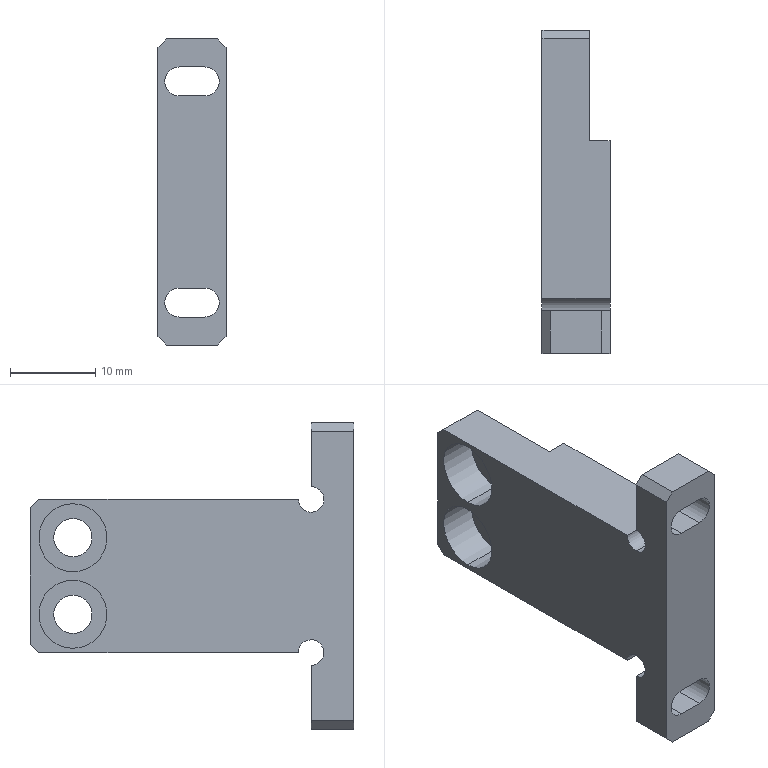Part | SolidWorks | features HoleWzd 2, ICE 2, Chamfer 1, Extrusion 1 | 1 solid | 39 faces | box 8 x 38 x 36 mm | volume 4843 mm3 | plane 24 | cylinder 15 | commonest cylinder face diameters 3.4 x4 4.5 x4 8 x4 3 x3
STEP:
#1=CARTESIAN_POINT('',(4.6,33.,-8.5));
#2=VERTEX_POINT('',#1);
#3=CARTESIAN_POINT('',(4.6,33.,-0.5));
#4=VERTEX_POINT('',#3);
#5=CARTESIAN_POINT('',(4.6,33.,-4.5));
#6=DIRECTION('',(-1.,0.,0.));
#7=DIRECTION('',(0.,0.,1.));
#8=AXIS2_PLACEMENT_3D('',#5,#6,#7);
#9=CIRCLE('',#8,4.);
#10=EDGE_CURVE('',#2,#4,#9,.T.);
#11=ORIENTED_EDGE('',*,*,#10,.F.);
#12=CARTESIAN_POINT('',(0.,33.,-8.5));
#13=VERTEX_POINT('',#12);
#14=CARTESIAN_POINT('',(0.,33.,-8.5));
#15=DIRECTION('',(-1.,0.,0.));
#16=VECTOR('',#15,1000.);
#17=LINE('',#14,#16);
#18=EDGE_CURVE('',#2,#13,#17,.T.);
#19=ORIENTED_EDGE('',*,*,#18,.T.);
#20=CARTESIAN_POINT('',(0.,33.,-0.5));
#21=VERTEX_POINT('',#20);
#22=CARTESIAN_POINT('',(0.,33.,-4.5));
#23=DIRECTION('',(-1.,0.,0.));
#24=DIRECTION('',(0.,0.,1.));
#25=AXIS2_PLACEMENT_3D('',#22,#23,#24);
#26=CIRCLE('',#25,4.);
#27=EDGE_CURVE('',#13,#21,#26,.T.);
#28=ORIENTED_EDGE('',*,*,#27,.T.);
#29=CARTESIAN_POINT('',(0.,33.,-0.5));
#30=DIRECTION('',(-1.,0.,0.));
#31=VECTOR('',#30,1000.);
#32=LINE('',#29,#31);
#33=EDGE_CURVE('',#4,#21,#32,.T.);
#34=ORIENTED_EDGE('',*,*,#33,.F.);
#35=EDGE_LOOP('',(#11,#19,#28,#34));
#36=FACE_OUTER_BOUND('',#35,.T.);
#37=CARTESIAN_POINT('',(0.,33.,-4.5));
#38=DIRECTION('',(-1.,0.,0.));
#39=DIRECTION('',(0.,0.,1.));
#40=AXIS2_PLACEMENT_3D('',#37,#38,#39);
#41=CYLINDRICAL_SURFACE('',#40,4.);
#42=ADVANCED_FACE('',(#36),#41,.F.);
#43=CARTESIAN_POINT('',(4.6,33.,0.5));
#44=VERTEX_POINT('',#43);
#45=CARTESIAN_POINT('',(4.6,33.,8.5));
#46=VERTEX_POINT('',#45);
#47=CARTESIAN_POINT('',(4.6,33.,4.5));
#48=DIRECTION('',(-1.,0.,0.));
#49=DIRECTION('',(0.,0.,1.));
#50=AXIS2_PLACEMENT_3D('',#47,#48,#49);
#51=CIRCLE('',#50,4.);
#52=EDGE_CURVE('',#44,#46,#51,.T.);
#53=ORIENTED_EDGE('',*,*,#52,.F.);
#54=CARTESIAN_POINT('',(0.,33.,0.5));
#55=VERTEX_POINT('',#54);
#56=CARTESIAN_POINT('',(0.,33.,0.5));
#57=DIRECTION('',(-1.,0.,0.));
#58=VECTOR('',#57,1000.);
#59=LINE('',#56,#58);
#60=EDGE_CURVE('',#44,#55,#59,.T.);
#61=ORIENTED_EDGE('',*,*,#60,.T.);
#62=CARTESIAN_POINT('',(0.,33.,8.5));
#63=VERTEX_POINT('',#62);
#64=CARTESIAN_POINT('',(0.,33.,4.5));
#65=DIRECTION('',(-1.,0.,0.));
#66=DIRECTION('',(0.,0.,1.));
#67=AXIS2_PLACEMENT_3D('',#64,#65,#66);
#68=CIRCLE('',#67,4.);
#69=EDGE_CURVE('',#55,#63,#68,.T.);
#70=ORIENTED_EDGE('',*,*,#69,.T.);
#71=CARTESIAN_POINT('',(0.,33.,8.5));
#72=DIRECTION('',(-1.,0.,0.));
#73=VECTOR('',#72,1000.);
#74=LINE('',#71,#73);
#75=EDGE_CURVE('',#46,#63,#74,.T.);
#76=ORIENTED_EDGE('',*,*,#75,.F.);
#77=EDGE_LOOP('',(#53,#61,#70,#76));
#78=FACE_OUTER_BOUND('',#77,.T.);
#79=CARTESIAN_POINT('',(0.,33.,4.5));
#80=DIRECTION('',(-1.,0.,0.));
#81=DIRECTION('',(0.,0.,1.));
#82=AXIS2_PLACEMENT_3D('',#79,#80,#81);
#83=CYLINDRICAL_SURFACE('',#82,4.);
#84=ADVANCED_FACE('',(#78),#83,.F.);
#85=CARTESIAN_POINT('',(0.,5.,7.5));
#86=VERTEX_POINT('',#85);
#87=CARTESIAN_POINT('',(0.,6.5,9.));
#88=VERTEX_POINT('',#87);
#89=CARTESIAN_POINT('',(0.,5.,9.));
#90=DIRECTION('',(1.,0.,0.));
#91=DIRECTION('',(0.,0.,-1.));
#92=AXIS2_PLACEMENT_3D('',#89,#90,#91);
#93=CIRCLE('',#92,1.5);
#94=EDGE_CURVE('',#86,#88,#93,.T.);
#95=ORIENTED_EDGE('',*,*,#94,.F.);
#96=CARTESIAN_POINT('',(8.,5.,7.5));
#97=VERTEX_POINT('',#96);
#98=CARTESIAN_POINT('',(0.,5.,7.5));
#99=DIRECTION('',(1.,0.,0.));
#100=VECTOR('',#99,1000.);
#101=LINE('',#98,#100);
#102=EDGE_CURVE('',#86,#97,#101,.T.);
#103=ORIENTED_EDGE('',*,*,#102,.T.);
#104=CARTESIAN_POINT('',(8.,6.5,9.));
#105=VERTEX_POINT('',#104);
#106=CARTESIAN_POINT('',(8.,5.,9.));
#107=DIRECTION('',(1.,0.,0.));
#108=DIRECTION('',(0.,0.,-1.));
#109=AXIS2_PLACEMENT_3D('',#106,#107,#108);
#110=CIRCLE('',#109,1.5);
#111=EDGE_CURVE('',#97,#105,#110,.T.);
#112=ORIENTED_EDGE('',*,*,#111,.T.);
#113=CARTESIAN_POINT('',(0.,6.5,9.));
#114=DIRECTION('',(1.,0.,0.));
#115=VECTOR('',#114,1000.);
#116=LINE('',#113,#115);
#117=EDGE_CURVE('',#88,#105,#116,.T.);
#118=ORIENTED_EDGE('',*,*,#117,.F.);
#119=EDGE_LOOP('',(#95,#103,#112,#118));
#120=FACE_OUTER_BOUND('',#119,.T.);
#121=CARTESIAN_POINT('',(0.,5.,9.));
#122=DIRECTION('',(1.,0.,0.));
#123=DIRECTION('',(0.,0.,-1.));
#124=AXIS2_PLACEMENT_3D('',#121,#122,#123);
#125=CYLINDRICAL_SURFACE('',#124,1.5);
#126=ADVANCED_FACE('',(#120),#125,.F.);
#127=CARTESIAN_POINT('',(5.6,33.,-6.75));
#128=VERTEX_POINT('',#127);
#129=CARTESIAN_POINT('',(5.6,33.,-2.25));
#130=VERTEX_POINT('',#129);
#131=CARTESIAN_POINT('',(5.6,33.,-4.5));
#132=DIRECTION('',(-1.,0.,0.));
#133=DIRECTION('',(0.,0.,-1.));
#134=AXIS2_PLACEMENT_3D('',#131,#132,#133);
#135=CIRCLE('',#134,2.25);
#136=EDGE_CURVE('',#128,#130,#135,.T.);
#137=ORIENTED_EDGE('',*,*,#136,.F.);
#138=CARTESIAN_POINT('',(4.6,33.,-6.75));
#139=VERTEX_POINT('',#138);
#140=CARTESIAN_POINT('',(0.,33.,-6.75));
#141=DIRECTION('',(-1.,0.,0.));
#142=VECTOR('',#141,1000.);
#143=LINE('',#140,#142);
#144=EDGE_CURVE('',#128,#139,#143,.T.);
#145=ORIENTED_EDGE('',*,*,#144,.T.);
#146=CARTESIAN_POINT('',(4.6,33.,-2.25));
#147=VERTEX_POINT('',#146);
#148=CARTESIAN_POINT('',(4.6,33.,-4.5));
#149=DIRECTION('',(-1.,0.,0.));
#150=DIRECTION('',(0.,0.,1.));
#151=AXIS2_PLACEMENT_3D('',#148,#149,#150);
#152=CIRCLE('',#151,2.25);
#153=EDGE_CURVE('',#139,#147,#152,.T.);
#154=ORIENTED_EDGE('',*,*,#153,.T.);
#155=CARTESIAN_POINT('',(0.,33.,-2.25));
#156=DIRECTION('',(-1.,0.,0.));
#157=VECTOR('',#156,1000.);
#158=LINE('',#155,#157);
#159=EDGE_CURVE('',#130,#147,#158,.T.);
#160=ORIENTED_EDGE('',*,*,#159,.F.);
#161=EDGE_LOOP('',(#137,#145,#154,#160));
#162=FACE_OUTER_BOUND('',#161,.T.);
#163=CARTESIAN_POINT('',(0.,33.,-4.5));
#164=DIRECTION('',(-1.,0.,0.));
#165=DIRECTION('',(0.,0.,1.));
#166=AXIS2_PLACEMENT_3D('',#163,#164,#165);
#167=CYLINDRICAL_SURFACE('',#166,2.25);
#168=ADVANCED_FACE('',(#162),#167,.F.);
#169=CARTESIAN_POINT('',(5.6,33.,2.25));
#170=VERTEX_POINT('',#169);
#171=CARTESIAN_POINT('',(5.6,33.,6.75));
#172=VERTEX_POINT('',#171);
#173=CARTESIAN_POINT('',(5.6,33.,4.5));
#174=DIRECTION('',(-1.,0.,0.));
#175=DIRECTION('',(0.,0.,-1.));
#176=AXIS2_PLACEMENT_3D('',#173,#174,#175);
#177=CIRCLE('',#176,2.25);
#178=EDGE_CURVE('',#170,#172,#177,.T.);
#179=ORIENTED_EDGE('',*,*,#178,.F.);
#180=CARTESIAN_POINT('',(4.6,33.,2.25));
#181=VERTEX_POINT('',#180);
#182=CARTESIAN_POINT('',(0.,33.,2.25));
#183=DIRECTION('',(-1.,0.,0.));
#184=VECTOR('',#183,1000.);
#185=LINE('',#182,#184);
#186=EDGE_CURVE('',#170,#181,#185,.T.);
#187=ORIENTED_EDGE('',*,*,#186,.T.);
#188=CARTESIAN_POINT('',(4.6,33.,6.75));
#189=VERTEX_POINT('',#188);
#190=CARTESIAN_POINT('',(4.6,33.,4.5));
#191=DIRECTION('',(-1.,0.,0.));
#192=DIRECTION('',(0.,0.,1.));
#193=AXIS2_PLACEMENT_3D('',#190,#191,#192);
#194=CIRCLE('',#193,2.25);
#195=EDGE_CURVE('',#181,#189,#194,.T.);
#196=ORIENTED_EDGE('',*,*,#195,.T.);
#197=CARTESIAN_POINT('',(0.,33.,6.75));
#198=DIRECTION('',(-1.,0.,0.));
#199=VECTOR('',#198,1000.);
#200=LINE('',#197,#199);
#201=EDGE_CURVE('',#172,#189,#200,.T.);
#202=ORIENTED_EDGE('',*,*,#201,.F.);
#203=EDGE_LOOP('',(#179,#187,#196,#202));
#204=FACE_OUTER_BOUND('',#203,.T.);
#205=CARTESIAN_POINT('',(0.,33.,4.5));
#206=DIRECTION('',(-1.,0.,0.));
#207=DIRECTION('',(0.,0.,1.));
#208=AXIS2_PLACEMENT_3D('',#205,#206,#207);
#209=CYLINDRICAL_SURFACE('',#208,2.25);
#210=ADVANCED_FACE('',(#204),#209,.F.);
#211=CARTESIAN_POINT('',(5.6,38.,-8.));
#212=VERTEX_POINT('',#211);
#213=CARTESIAN_POINT('',(5.6,38.,8.));
#214=VERTEX_POINT('',#213);
#215=CARTESIAN_POINT('',(5.6,38.,9.));
#216=DIRECTION('',(0.,0.,1.));
#217=VECTOR('',#216,1000.);
#218=LINE('',#215,#217);
#219=EDGE_CURVE('',#212,#214,#218,.T.);
#220=ORIENTED_EDGE('',*,*,#219,.F.);
#221=CARTESIAN_POINT('',(0.,38.,-8.));
#222=VERTEX_POINT('',#221);
#223=CARTESIAN_POINT('',(8.,38.,-8.));
#224=DIRECTION('',(-1.,0.,0.));
#225=VECTOR('',#224,1000.);
#226=LINE('',#223,#225);
#227=EDGE_CURVE('',#212,#222,#226,.T.);
#228=ORIENTED_EDGE('',*,*,#227,.T.);
#229=CARTESIAN_POINT('',(0.,38.,8.));
#230=VERTEX_POINT('',#229);
#231=CARTESIAN_POINT('',(0.,38.,9.));
#232=DIRECTION('',(0.,0.,1.));
#233=VECTOR('',#232,1000.);
#234=LINE('',#231,#233);
#235=EDGE_CURVE('',#222,#230,#234,.T.);
#236=ORIENTED_EDGE('',*,*,#235,.T.);
#237=CARTESIAN_POINT('',(8.,38.,8.));
#238=DIRECTION('',(1.,0.,0.));
#239=VECTOR('',#238,1000.);
#240=LINE('',#237,#239);
#241=EDGE_CURVE('',#230,#214,#240,.T.);
#242=ORIENTED_EDGE('',*,*,#241,.T.);
#243=EDGE_LOOP('',(#220,#228,#236,#242));
#244=FACE_OUTER_BOUND('',#243,.T.);
#245=CARTESIAN_POINT('',(8.,38.,9.));
#246=DIRECTION('',(0.,-1.,0.));
#247=DIRECTION('',(0.,0.,-1.));
#248=AXIS2_PLACEMENT_3D('',#245,#246,#247);
#249=PLANE('',#248);
#250=ADVANCED_FACE('',(#244),#249,.F.);
#251=ORIENTED_EDGE('',*,*,#186,.F.);
#252=CARTESIAN_POINT('',(5.6,33.,4.5));
#253=DIRECTION('',(-1.,0.,0.));
#254=DIRECTION('',(0.,0.,-1.));
#255=AXIS2_PLACEMENT_3D('',#252,#253,#254);
#256=CIRCLE('',#255,2.25);
#257=EDGE_CURVE('',#172,#170,#256,.T.);
#258=ORIENTED_EDGE('',*,*,#257,.F.);
#259=ORIENTED_EDGE('',*,*,#201,.T.);
#260=CARTESIAN_POINT('',(4.6,33.,4.5));
#261=DIRECTION('',(-1.,0.,0.));
#262=DIRECTION('',(0.,0.,1.));
#263=AXIS2_PLACEMENT_3D('',#260,#261,#262);
#264=CIRCLE('',#263,2.25);
#265=EDGE_CURVE('',#189,#181,#264,.T.);
#266=ORIENTED_EDGE('',*,*,#265,.T.);
#267=EDGE_LOOP('',(#251,#258,#259,#266));
#268=FACE_OUTER_BOUND('',#267,.T.);
#269=CARTESIAN_POINT('',(0.,33.,4.5));
#270=DIRECTION('',(-1.,0.,0.));
#271=DIRECTION('',(0.,0.,1.));
#272=AXIS2_PLACEMENT_3D('',#269,#270,#271);
#273=CYLINDRICAL_SURFACE('',#272,2.25);
#274=ADVANCED_FACE('',(#268),#273,.F.);
#275=ORIENTED_EDGE('',*,*,#144,.F.);
#276=CARTESIAN_POINT('',(5.6,33.,-4.5));
#277=DIRECTION('',(-1.,0.,0.));
#278=DIRECTION('',(0.,0.,-1.));
#279=AXIS2_PLACEMENT_3D('',#276,#277,#278);
#280=CIRCLE('',#279,2.25);
#281=EDGE_CURVE('',#130,#128,#280,.T.);
#282=ORIENTED_EDGE('',*,*,#281,.F.);
#283=ORIENTED_EDGE('',*,*,#159,.T.);
#284=CARTESIAN_POINT('',(4.6,33.,-4.5));
#285=DIRECTION('',(-1.,0.,0.));
#286=DIRECTION('',(0.,0.,1.));
#287=AXIS2_PLACEMENT_3D('',#284,#285,#286);
#288=CIRCLE('',#287,2.25);
#289=EDGE_CURVE('',#147,#139,#288,.T.);
#290=ORIENTED_EDGE('',*,*,#289,.T.);
#291=EDGE_LOOP('',(#275,#282,#283,#290));
#292=FACE_OUTER_BOUND('',#291,.T.);
#293=CARTESIAN_POINT('',(0.,33.,-4.5));
#294=DIRECTION('',(-1.,0.,0.));
#295=DIRECTION('',(0.,0.,1.));
#296=AXIS2_PLACEMENT_3D('',#293,#294,#295);
#297=CYLINDRICAL_SURFACE('',#296,2.25);
#298=ADVANCED_FACE('',(#292),#297,.F.);
#299=CARTESIAN_POINT('',(5.6,37.,9.));
#300=VERTEX_POINT('',#299);
#301=CARTESIAN_POINT('',(0.,37.,9.));
#302=VERTEX_POINT('',#301);
#303=CARTESIAN_POINT('',(8.,37.,9.));
#304=DIRECTION('',(-1.,0.,0.));
#305=VECTOR('',#304,1000.);
#306=LINE('',#303,#305);
#307=EDGE_CURVE('',#300,#302,#306,.T.);
#308=ORIENTED_EDGE('',*,*,#307,.F.);
#309=CARTESIAN_POINT('',(5.6,37.,9.));
#310=DIRECTION('',(0.,0.7071,-0.7071));
#311=VECTOR('',#310,1000.);
#312=LINE('',#309,#311);
#313=EDGE_CURVE('',#300,#214,#312,.T.);
#314=ORIENTED_EDGE('',*,*,#313,.T.);
#315=ORIENTED_EDGE('',*,*,#241,.F.);
#316=CARTESIAN_POINT('',(0.,37.,9.));
#317=DIRECTION('',(0.,0.7071,-0.7071));
#318=VECTOR('',#317,1000.);
#319=LINE('',#316,#318);
#320=EDGE_CURVE('',#302,#230,#319,.T.);
#321=ORIENTED_EDGE('',*,*,#320,.F.);
#322=EDGE_LOOP('',(#308,#314,#315,#321));
#323=FACE_OUTER_BOUND('',#322,.T.);
#324=CARTESIAN_POINT('',(8.,37.,9.));
#325=DIRECTION('',(0.,-0.7071,-0.7071));
#326=DIRECTION('',(-1.,0.,0.));
#327=AXIS2_PLACEMENT_3D('',#324,#325,#326);
#328=PLANE('',#327);
#329=ADVANCED_FACE('',(#323),#328,.F.);
#330=ORIENTED_EDGE('',*,*,#227,.F.);
#331=CARTESIAN_POINT('',(5.6,37.,-9.));
#332=VERTEX_POINT('',#331);
#333=CARTESIAN_POINT('',(5.6,38.,-8.));
#334=DIRECTION('',(0.,-0.7071,-0.7071));
#335=VECTOR('',#334,1000.);
#336=LINE('',#333,#335);
#337=EDGE_CURVE('',#212,#332,#336,.T.);
#338=ORIENTED_EDGE('',*,*,#337,.T.);
#339=CARTESIAN_POINT('',(0.,37.,-9.));
#340=VERTEX_POINT('',#339);
#341=CARTESIAN_POINT('',(8.,37.,-9.));
#342=DIRECTION('',(1.,0.,0.));
#343=VECTOR('',#342,1000.);
#344=LINE('',#341,#343);
#345=EDGE_CURVE('',#340,#332,#344,.T.);
#346=ORIENTED_EDGE('',*,*,#345,.F.);
#347=CARTESIAN_POINT('',(0.,38.,-8.));
#348=DIRECTION('',(0.,-0.7071,-0.7071));
#349=VECTOR('',#348,1000.);
#350=LINE('',#347,#349);
#351=EDGE_CURVE('',#222,#340,#350,.T.);
#352=ORIENTED_EDGE('',*,*,#351,.F.);
#353=EDGE_LOOP('',(#330,#338,#346,#352));
#354=FACE_OUTER_BOUND('',#353,.T.);
#355=CARTESIAN_POINT('',(8.,38.,-8.));
#356=DIRECTION('',(0.,-0.7071,0.7071));
#357=DIRECTION('',(-1.,0.,0.));
#358=AXIS2_PLACEMENT_3D('',#355,#356,#357);
#359=PLANE('',#358);
#360=ADVANCED_FACE('',(#354),#359,.F.);
#361=CARTESIAN_POINT('',(7.,5.,18.));
#362=VERTEX_POINT('',#361);
#363=CARTESIAN_POINT('',(1.,5.,18.));
#364=VERTEX_POINT('',#363);
#365=CARTESIAN_POINT('',(8.,5.,18.));
#366=DIRECTION('',(-1.,0.,0.));
#367=VECTOR('',#366,1000.);
#368=LINE('',#365,#367);
#369=EDGE_CURVE('',#362,#364,#368,.T.);
#370=ORIENTED_EDGE('',*,*,#369,.F.);
#371=CARTESIAN_POINT('',(8.,5.,17.));
#372=VERTEX_POINT('',#371);
#373=CARTESIAN_POINT('',(8.,5.,17.));
#374=DIRECTION('',(0.7071,0.,-0.7071));
#375=VECTOR('',#374,1000.);
#376=LINE('',#373,#375);
#377=EDGE_CURVE('',#362,#372,#376,.T.);
#378=ORIENTED_EDGE('',*,*,#377,.T.);
#379=CARTESIAN_POINT('',(8.,5.,10.5));
#380=VERTEX_POINT('',#379);
#381=CARTESIAN_POINT('',(8.,5.,9.));
#382=DIRECTION('',(0.,0.,1.));
#383=VECTOR('',#382,1000.);
#384=LINE('',#381,#383);
#385=EDGE_CURVE('',#380,#372,#384,.T.);
#386=ORIENTED_EDGE('',*,*,#385,.F.);
#387=CARTESIAN_POINT('',(0.,5.,10.5));
#388=VERTEX_POINT('',#387);
#389=CARTESIAN_POINT('',(0.,5.,10.5));
#390=DIRECTION('',(-1.,0.,0.));
#391=VECTOR('',#390,1000.);
#392=LINE('',#389,#391);
#393=EDGE_CURVE('',#380,#388,#392,.T.);
#394=ORIENTED_EDGE('',*,*,#393,.T.);
#395=CARTESIAN_POINT('',(0.,5.,17.));
#396=VERTEX_POINT('',#395);
#397=CARTESIAN_POINT('',(0.,5.,9.));
#398=DIRECTION('',(0.,0.,1.));
#399=VECTOR('',#398,1000.);
#400=LINE('',#397,#399);
#401=EDGE_CURVE('',#388,#396,#400,.T.);
#402=ORIENTED_EDGE('',*,*,#401,.T.);
#403=CARTESIAN_POINT('',(1.,5.,18.));
#404=DIRECTION('',(0.7071,0.,0.7071));
#405=VECTOR('',#404,1000.);
#406=LINE('',#403,#405);
#407=EDGE_CURVE('',#396,#364,#406,.T.);
#408=ORIENTED_EDGE('',*,*,#407,.T.);
#409=EDGE_LOOP('',(#370,#378,#386,#394,#402,#408));
#410=FACE_OUTER_BOUND('',#409,.T.);
#411=CARTESIAN_POINT('',(2.5,5.,11.3));
#412=VERTEX_POINT('',#411);
#413=CARTESIAN_POINT('',(2.5,5.,14.7));
#414=VERTEX_POINT('',#413);
#415=CARTESIAN_POINT('',(2.5,5.,13.));
#416=DIRECTION('',(0.,1.,0.));
#417=DIRECTION('',(0.,0.,1.));
#418=AXIS2_PLACEMENT_3D('',#415,#416,#417);
#419=CIRCLE('',#418,1.7);
#420=EDGE_CURVE('',#412,#414,#419,.T.);
#421=ORIENTED_EDGE('',*,*,#420,.F.);
#422=CARTESIAN_POINT('',(5.5,5.,11.3));
#423=VERTEX_POINT('',#422);
#424=CARTESIAN_POINT('',(2.5,5.,11.3));
#425=DIRECTION('',(1.,0.,0.));
#426=VECTOR('',#425,1000.);
#427=LINE('',#424,#426);
#428=EDGE_CURVE('',#412,#423,#427,.T.);
#429=ORIENTED_EDGE('',*,*,#428,.T.);
#430=CARTESIAN_POINT('',(5.5,5.,14.7));
#431=VERTEX_POINT('',#430);
#432=CARTESIAN_POINT('',(5.5,5.,13.));
#433=DIRECTION('',(0.,1.,0.));
#434=DIRECTION('',(0.,0.,1.));
#435=AXIS2_PLACEMENT_3D('',#432,#433,#434);
#436=CIRCLE('',#435,1.7);
#437=EDGE_CURVE('',#431,#423,#436,.T.);
#438=ORIENTED_EDGE('',*,*,#437,.F.);
#439=CARTESIAN_POINT('',(2.5,5.,14.7));
#440=DIRECTION('',(1.,0.,0.));
#441=VECTOR('',#440,1000.);
#442=LINE('',#439,#441);
#443=EDGE_CURVE('',#414,#431,#442,.T.);
#444=ORIENTED_EDGE('',*,*,#443,.F.);
#445=EDGE_LOOP('',(#421,#429,#438,#444));
#446=FACE_BOUND('',#445,.T.);
#447=CARTESIAN_POINT('',(8.,5.,9.));
#448=DIRECTION('',(0.,-1.,0.));
#449=DIRECTION('',(0.,0.,-1.));
#450=AXIS2_PLACEMENT_3D('',#447,#448,#449);
#451=PLANE('',#450);
#452=ADVANCED_FACE('',(#410,#446),#451,.F.);
#453=CARTESIAN_POINT('',(5.6,25.,-9.));
#454=VERTEX_POINT('',#453);
#455=CARTESIAN_POINT('',(5.6,38.,-9.));
#456=DIRECTION('',(0.,1.,0.));
#457=VECTOR('',#456,1000.);
#458=LINE('',#455,#457);
#459=EDGE_CURVE('',#454,#332,#458,.T.);
#460=ORIENTED_EDGE('',*,*,#459,.F.);
#461=CARTESIAN_POINT('',(8.,25.,-9.));
#462=VERTEX_POINT('',#461);
#463=CARTESIAN_POINT('',(5.6,25.,-9.));
#464=DIRECTION('',(1.,0.,0.));
#465=VECTOR('',#464,1000.);
#466=LINE('',#463,#465);
#467=EDGE_CURVE('',#454,#462,#466,.T.);
#468=ORIENTED_EDGE('',*,*,#467,.T.);
#469=CARTESIAN_POINT('',(8.,6.5,-9.));
#470=VERTEX_POINT('',#469);
#471=CARTESIAN_POINT('',(8.,38.,-9.));
#472=DIRECTION('',(0.,1.,0.));
#473=VECTOR('',#472,1000.);
#474=LINE('',#471,#473);
#475=EDGE_CURVE('',#470,#462,#474,.T.);
#476=ORIENTED_EDGE('',*,*,#475,.F.);
#477=CARTESIAN_POINT('',(0.,6.5,-9.));
#478=VERTEX_POINT('',#477);
#479=CARTESIAN_POINT('',(0.,6.5,-9.));
#480=DIRECTION('',(-1.,0.,0.));
#481=VECTOR('',#480,1000.);
#482=LINE('',#479,#481);
#483=EDGE_CURVE('',#470,#478,#482,.T.);
#484=ORIENTED_EDGE('',*,*,#483,.T.);
#485=CARTESIAN_POINT('',(0.,38.,-9.));
#486=DIRECTION('',(0.,1.,0.));
#487=VECTOR('',#486,1000.);
#488=LINE('',#485,#487);
#489=EDGE_CURVE('',#478,#340,#488,.T.);
#490=ORIENTED_EDGE('',*,*,#489,.T.);
#491=ORIENTED_EDGE('',*,*,#345,.T.);
#492=EDGE_LOOP('',(#460,#468,#476,#484,#490,#491));
#493=FACE_OUTER_BOUND('',#492,.T.);
#494=CARTESIAN_POINT('',(8.,38.,-9.));
#495=DIRECTION('',(0.,0.,1.));
#496=DIRECTION('',(0.,-1.,0.));
#497=AXIS2_PLACEMENT_3D('',#494,#495,#496);
#498=PLANE('',#497);
#499=ADVANCED_FACE('',(#493),#498,.F.);
#500=CARTESIAN_POINT('',(8.,25.,9.));
#501=VERTEX_POINT('',#500);
#502=CARTESIAN_POINT('',(8.,38.,9.));
#503=DIRECTION('',(0.,-1.,0.));
#504=VECTOR('',#503,1000.);
#505=LINE('',#502,#504);
#506=EDGE_CURVE('',#501,#105,#505,.T.);
#507=ORIENTED_EDGE('',*,*,#506,.F.);
#508=CARTESIAN_POINT('',(5.6,25.,9.));
#509=VERTEX_POINT('',#508);
#510=CARTESIAN_POINT('',(5.6,25.,9.));
#511=DIRECTION('',(1.,0.,0.));
#512=VECTOR('',#511,1000.);
#513=LINE('',#510,#512);
#514=EDGE_CURVE('',#509,#501,#513,.T.);
#515=ORIENTED_EDGE('',*,*,#514,.F.);
#516=CARTESIAN_POINT('',(5.6,38.,9.));
#517=DIRECTION('',(0.,-1.,0.));
#518=VECTOR('',#517,1000.);
#519=LINE('',#516,#518);
#520=EDGE_CURVE('',#300,#509,#519,.T.);
#521=ORIENTED_EDGE('',*,*,#520,.F.);
#522=ORIENTED_EDGE('',*,*,#307,.T.);
#523=CARTESIAN_POINT('',(0.,38.,9.));
#524=DIRECTION('',(0.,-1.,0.));
#525=VECTOR('',#524,1000.);
#526=LINE('',#523,#525);
#527=EDGE_CURVE('',#302,#88,#526,.T.);
#528=ORIENTED_EDGE('',*,*,#527,.T.);
#529=ORIENTED_EDGE('',*,*,#117,.T.);
#530=EDGE_LOOP('',(#507,#515,#521,#522,#528,#529));
#531=FACE_OUTER_BOUND('',#530,.T.);
#532=CARTESIAN_POINT('',(8.,38.,9.));
#533=DIRECTION('',(0.,0.,-1.));
#534=DIRECTION('',(0.,1.,0.));
#535=AXIS2_PLACEMENT_3D('',#532,#533,#534);
#536=PLANE('',#535);
#537=ADVANCED_FACE('',(#531),#536,.F.);
#538=CARTESIAN_POINT('',(7.,0.,18.));
#539=VERTEX_POINT('',#538);
#540=CARTESIAN_POINT('',(1.,0.,18.));
#541=VERTEX_POINT('',#540);
#542=CARTESIAN_POINT('',(8.,0.,18.));
#543=DIRECTION('',(-1.,0.,0.));
#544=VECTOR('',#543,1000.);
#545=LINE('',#542,#544);
#546=EDGE_CURVE('',#539,#541,#545,.T.);
#547=ORIENTED_EDGE('',*,*,#546,.F.);
#548=CARTESIAN_POINT('',(7.,5.,18.));
#549=DIRECTION('',(0.,1.,0.));
#550=VECTOR('',#549,1000.);
#551=LINE('',#548,#550);
#552=EDGE_CURVE('',#539,#362,#551,.T.);
#553=ORIENTED_EDGE('',*,*,#552,.T.);
#554=ORIENTED_EDGE('',*,*,#369,.T.);
#555=CARTESIAN_POINT('',(1.,5.,18.));
#556=DIRECTION('',(0.,-1.,0.));
#557=VECTOR('',#556,1000.);
#558=LINE('',#555,#557);
#559=EDGE_CURVE('',#364,#541,#558,.T.);
#560=ORIENTED_EDGE('',*,*,#559,.T.);
#561=EDGE_LOOP('',(#547,#553,#554,#560));
#562=FACE_OUTER_BOUND('',#561,.T.);
#563=CARTESIAN_POINT('',(8.,5.,18.));
#564=DIRECTION('',(0.,0.,-1.));
#565=DIRECTION('',(-1.,0.,0.));
#566=AXIS2_PLACEMENT_3D('',#563,#564,#565);
#567=PLANE('',#566);
#568=ADVANCED_FACE('',(#562),#567,.F.);
#569=CARTESIAN_POINT('',(2.5,0.,-11.3));
#570=VERTEX_POINT('',#569);
#571=CARTESIAN_POINT('',(5.5,0.,-11.3));
#572=VERTEX_POINT('',#571);
#573=CARTESIAN_POINT('',(2.5,0.,-11.3));
#574=DIRECTION('',(1.,0.,0.));
#575=VECTOR('',#574,1000.);
#576=LINE('',#573,#575);
#577=EDGE_CURVE('',#570,#572,#576,.T.);
#578=ORIENTED_EDGE('',*,*,#577,.T.);
#579=CARTESIAN_POINT('',(5.5,0.,-14.7));
#580=VERTEX_POINT('',#579);
#581=CARTESIAN_POINT('',(5.5,0.,-13.));
#582=DIRECTION('',(0.,1.,0.));
#583=DIRECTION('',(0.,0.,1.));
#584=AXIS2_PLACEMENT_3D('',#581,#582,#583);
#585=CIRCLE('',#584,1.7);
#586=EDGE_CURVE('',#572,#580,#585,.T.);
#587=ORIENTED_EDGE('',*,*,#586,.T.);
#588=CARTESIAN_POINT('',(2.5,0.,-14.7));
#589=VERTEX_POINT('',#588);
#590=CARTESIAN_POINT('',(2.5,0.,-14.7));
#591=DIRECTION('',(1.,0.,0.));
#592=VECTOR('',#591,1000.);
#593=LINE('',#590,#592);
#594=EDGE_CURVE('',#589,#580,#593,.T.);
#595=ORIENTED_EDGE('',*,*,#594,.F.);
#596=CARTESIAN_POINT('',(2.5,0.,-13.));
#597=DIRECTION('',(0.,1.,0.));
#598=DIRECTION('',(0.,0.,1.));
#599=AXIS2_PLACEMENT_3D('',#596,#597,#598);
#600=CIRCLE('',#599,1.7);
#601=EDGE_CURVE('',#589,#570,#600,.T.);
#602=ORIENTED_EDGE('',*,*,#601,.T.);
#603=EDGE_LOOP('',(#578,#587,#595,#602));
#604=FACE_BOUND('',#603,.T.);
#605=CARTESIAN_POINT('',(2.5,0.,11.3));
#606=VERTEX_POINT('',#605);
#607=CARTESIAN_POINT('',(2.5,0.,14.7));
#608=VERTEX_POINT('',#607);
#609=CARTESIAN_POINT('',(2.5,0.,13.));
#610=DIRECTION('',(0.,1.,0.));
#611=DIRECTION('',(0.,0.,1.));
#612=AXIS2_PLACEMENT_3D('',#609,#610,#611);
#613=CIRCLE('',#612,1.7);
#614=EDGE_CURVE('',#606,#608,#613,.T.);
#615=ORIENTED_EDGE('',*,*,#614,.T.);
#616=CARTESIAN_POINT('',(5.5,0.,14.7));
#617=VERTEX_POINT('',#616);
#618=CARTESIAN_POINT('',(2.5,0.,14.7));
#619=DIRECTION('',(1.,0.,0.));
#620=VECTOR('',#619,1000.);
#621=LINE('',#618,#620);
#622=EDGE_CURVE('',#608,#617,#621,.T.);
#623=ORIENTED_EDGE('',*,*,#622,.T.);
#624=CARTESIAN_POINT('',(5.5,0.,11.3));
#625=VERTEX_POINT('',#624);
#626=CARTESIAN_POINT('',(5.5,0.,13.));
#627=DIRECTION('',(0.,1.,0.));
#628=DIRECTION('',(0.,0.,1.));
#629=AXIS2_PLACEMENT_3D('',#626,#627,#628);
#630=CIRCLE('',#629,1.7);
#631=EDGE_CURVE('',#617,#625,#630,.T.);
#632=ORIENTED_EDGE('',*,*,#631,.T.);
#633=CARTESIAN_POINT('',(2.5,0.,11.3));
#634=DIRECTION('',(1.,0.,0.));
#635=VECTOR('',#634,1000.);
#636=LINE('',#633,#635);
#637=EDGE_CURVE('',#606,#625,#636,.T.);
#638=ORIENTED_EDGE('',*,*,#637,.F.);
#639=EDGE_LOOP('',(#615,#623,#632,#638));
#640=FACE_BOUND('',#639,.T.);
#641=CARTESIAN_POINT('',(7.,0.,-18.));
#642=VERTEX_POINT('',#641);
#643=CARTESIAN_POINT('',(1.,0.,-18.));
#644=VERTEX_POINT('',#643);
#645=CARTESIAN_POINT('',(8.,0.,-18.));
#646=DIRECTION('',(-1.,0.,0.));
#647=VECTOR('',#646,1000.);
#648=LINE('',#645,#647);
#649=EDGE_CURVE('',#642,#644,#648,.T.);
#650=ORIENTED_EDGE('',*,*,#649,.F.);
#651=CARTESIAN_POINT('',(8.,0.,-17.));
#652=VERTEX_POINT('',#651);
#653=CARTESIAN_POINT('',(8.,0.,-17.));
#654=DIRECTION('',(0.7071,0.,0.7071));
#655=VECTOR('',#654,1000.);
#656=LINE('',#653,#655);
#657=EDGE_CURVE('',#642,#652,#656,.T.);
#658=ORIENTED_EDGE('',*,*,#657,.T.);
#659=CARTESIAN_POINT('',(8.,0.,17.));
#660=VERTEX_POINT('',#659);
#661=CARTESIAN_POINT('',(8.,0.,-18.));
#662=DIRECTION('',(0.,0.,-1.));
#663=VECTOR('',#662,1000.);
#664=LINE('',#661,#663);
#665=EDGE_CURVE('',#660,#652,#664,.T.);
#666=ORIENTED_EDGE('',*,*,#665,.F.);
#667=CARTESIAN_POINT('',(8.,0.,17.));
#668=DIRECTION('',(-0.7071,0.,0.7071));
#669=VECTOR('',#668,1000.);
#670=LINE('',#667,#669);
#671=EDGE_CURVE('',#660,#539,#670,.T.);
#672=ORIENTED_EDGE('',*,*,#671,.T.);
#673=ORIENTED_EDGE('',*,*,#546,.T.);
#674=CARTESIAN_POINT('',(0.,0.,17.));
#675=VERTEX_POINT('',#674);
#676=CARTESIAN_POINT('',(1.,0.,18.));
#677=DIRECTION('',(-0.7071,0.,-0.7071));
#678=VECTOR('',#677,1000.);
#679=LINE('',#676,#678);
#680=EDGE_CURVE('',#541,#675,#679,.T.);
#681=ORIENTED_EDGE('',*,*,#680,.T.);
#682=CARTESIAN_POINT('',(0.,0.,-17.));
#683=VERTEX_POINT('',#682);
#684=CARTESIAN_POINT('',(0.,0.,-18.));
#685=DIRECTION('',(0.,0.,-1.));
#686=VECTOR('',#685,1000.);
#687=LINE('',#684,#686);
#688=EDGE_CURVE('',#675,#683,#687,.T.);
#689=ORIENTED_EDGE('',*,*,#688,.T.);
#690=CARTESIAN_POINT('',(1.,0.,-18.));
#691=DIRECTION('',(0.7071,0.,-0.7071));
#692=VECTOR('',#691,1000.);
#693=LINE('',#690,#692);
#694=EDGE_CURVE('',#683,#644,#693,.T.);
#695=ORIENTED_EDGE('',*,*,#694,.T.);
#696=EDGE_LOOP('',(#650,#658,#666,#672,#673,#681,#689,#695));
#697=FACE_OUTER_BOUND('',#696,.T.);
#698=CARTESIAN_POINT('',(8.,0.,-18.));
#699=DIRECTION('',(0.,1.,0.));
#700=DIRECTION('',(0.,0.,1.));
#701=AXIS2_PLACEMENT_3D('',#698,#699,#700);
#702=PLANE('',#701);
#703=ADVANCED_FACE('',(#604,#640,#697),#702,.F.);
#704=CARTESIAN_POINT('',(7.,5.,-18.));
#705=VERTEX_POINT('',#704);
#706=CARTESIAN_POINT('',(1.,5.,-18.));
#707=VERTEX_POINT('',#706);
#708=CARTESIAN_POINT('',(8.,5.,-18.));
#709=DIRECTION('',(-1.,0.,0.));
#710=VECTOR('',#709,1000.);
#711=LINE('',#708,#710);
#712=EDGE_CURVE('',#705,#707,#711,.T.);
#713=ORIENTED_EDGE('',*,*,#712,.F.);
#714=CARTESIAN_POINT('',(7.,0.,-18.));
#715=DIRECTION('',(0.,-1.,0.));
#716=VECTOR('',#715,1000.);
#717=LINE('',#714,#716);
#718=EDGE_CURVE('',#705,#642,#717,.T.);
#719=ORIENTED_EDGE('',*,*,#718,.T.);
#720=ORIENTED_EDGE('',*,*,#649,.T.);
#721=CARTESIAN_POINT('',(1.,5.,-18.));
#722=DIRECTION('',(0.,1.,0.));
#723=VECTOR('',#722,1000.);
#724=LINE('',#721,#723);
#725=EDGE_CURVE('',#644,#707,#724,.T.);
#726=ORIENTED_EDGE('',*,*,#725,.T.);
#727=EDGE_LOOP('',(#713,#719,#720,#726));
#728=FACE_OUTER_BOUND('',#727,.T.);
#729=CARTESIAN_POINT('',(8.,5.,-18.));
#730=DIRECTION('',(0.,0.,1.));
#731=DIRECTION('',(1.,0.,0.));
#732=AXIS2_PLACEMENT_3D('',#729,#730,#731);
#733=PLANE('',#732);
#734=ADVANCED_FACE('',(#728),#733,.F.);
#735=CARTESIAN_POINT('',(2.5,5.,-14.7));
#736=VERTEX_POINT('',#735);
#737=CARTESIAN_POINT('',(2.5,5.,-11.3));
#738=VERTEX_POINT('',#737);
#739=CARTESIAN_POINT('',(2.5,5.,-13.));
#740=DIRECTION('',(0.,1.,0.));
#741=DIRECTION('',(0.,0.,1.));
#742=AXIS2_PLACEMENT_3D('',#739,#740,#741);
#743=CIRCLE('',#742,1.7);
#744=EDGE_CURVE('',#736,#738,#743,.T.);
#745=ORIENTED_EDGE('',*,*,#744,.F.);
#746=CARTESIAN_POINT('',(5.5,5.,-14.7));
#747=VERTEX_POINT('',#746);
#748=CARTESIAN_POINT('',(2.5,5.,-14.7));
#749=DIRECTION('',(1.,0.,0.));
#750=VECTOR('',#749,1000.);
#751=LINE('',#748,#750);
#752=EDGE_CURVE('',#736,#747,#751,.T.);
#753=ORIENTED_EDGE('',*,*,#752,.T.);
#754=CARTESIAN_POINT('',(5.5,5.,-11.3));
#755=VERTEX_POINT('',#754);
#756=CARTESIAN_POINT('',(5.5,5.,-13.));
#757=DIRECTION('',(0.,1.,0.));
#758=DIRECTION('',(0.,0.,1.));
#759=AXIS2_PLACEMENT_3D('',#756,#757,#758);
#760=CIRCLE('',#759,1.7);
#761=EDGE_CURVE('',#755,#747,#760,.T.);
#762=ORIENTED_EDGE('',*,*,#761,.F.);
#763=CARTESIAN_POINT('',(2.5,5.,-11.3));
#764=DIRECTION('',(1.,0.,0.));
#765=VECTOR('',#764,1000.);
#766=LINE('',#763,#765);
#767=EDGE_CURVE('',#738,#755,#766,.T.);
#768=ORIENTED_EDGE('',*,*,#767,.F.);
#769=EDGE_LOOP('',(#745,#753,#762,#768));
#770=FACE_BOUND('',#769,.T.);
#771=CARTESIAN_POINT('',(8.,5.,-17.));
#772=VERTEX_POINT('',#771);
#773=CARTESIAN_POINT('',(8.,5.,-10.5));
#774=VERTEX_POINT('',#773);
#775=CARTESIAN_POINT('',(8.,5.,-9.));
#776=DIRECTION('',(0.,0.,1.));
#777=VECTOR('',#776,1000.);
#778=LINE('',#775,#777);
#779=EDGE_CURVE('',#772,#774,#778,.T.);
#780=ORIENTED_EDGE('',*,*,#779,.F.);
#781=CARTESIAN_POINT('',(8.,5.,-17.));
#782=DIRECTION('',(-0.7071,0.,-0.7071));
#783=VECTOR('',#782,1000.);
#784=LINE('',#781,#783);
#785=EDGE_CURVE('',#772,#705,#784,.T.);
#786=ORIENTED_EDGE('',*,*,#785,.T.);
#787=ORIENTED_EDGE('',*,*,#712,.T.);
#788=CARTESIAN_POINT('',(0.,5.,-17.));
#789=VERTEX_POINT('',#788);
#790=CARTESIAN_POINT('',(1.,5.,-18.));
#791=DIRECTION('',(-0.7071,0.,0.7071));
#792=VECTOR('',#791,1000.);
#793=LINE('',#790,#792);
#794=EDGE_CURVE('',#707,#789,#793,.T.);
#795=ORIENTED_EDGE('',*,*,#794,.T.);
#796=CARTESIAN_POINT('',(0.,5.,-10.5));
#797=VERTEX_POINT('',#796);
#798=CARTESIAN_POINT('',(0.,5.,-9.));
#799=DIRECTION('',(0.,0.,1.));
#800=VECTOR('',#799,1000.);
#801=LINE('',#798,#800);
#802=EDGE_CURVE('',#789,#797,#801,.T.);
#803=ORIENTED_EDGE('',*,*,#802,.T.);
#804=CARTESIAN_POINT('',(0.,5.,-10.5));
#805=DIRECTION('',(1.,0.,0.));
#806=VECTOR('',#805,1000.);
#807=LINE('',#804,#806);
#808=EDGE_CURVE('',#797,#774,#807,.T.);
#809=ORIENTED_EDGE('',*,*,#808,.T.);
#810=EDGE_LOOP('',(#780,#786,#787,#795,#803,#809));
#811=FACE_OUTER_BOUND('',#810,.T.);
#812=CARTESIAN_POINT('',(8.,5.,-9.));
#813=DIRECTION('',(0.,-1.,0.));
#814=DIRECTION('',(0.,0.,-1.));
#815=AXIS2_PLACEMENT_3D('',#812,#813,#814);
#816=PLANE('',#815);
#817=ADVANCED_FACE('',(#770,#811),#816,.F.);
#818=CARTESIAN_POINT('',(8.,25.,9.));
#819=DIRECTION('',(0.,0.,-1.));
#820=VECTOR('',#819,1000.);
#821=LINE('',#818,#820);
#822=EDGE_CURVE('',#501,#462,#821,.T.);
#823=ORIENTED_EDGE('',*,*,#822,.F.);
#824=ORIENTED_EDGE('',*,*,#506,.T.);
#825=ORIENTED_EDGE('',*,*,#111,.F.);
#826=CARTESIAN_POINT('',(8.,5.,9.));
#827=DIRECTION('',(1.,0.,0.));
#828=DIRECTION('',(0.,0.,-1.));
#829=AXIS2_PLACEMENT_3D('',#826,#827,#828);
#830=CIRCLE('',#829,1.5);
#831=EDGE_CURVE('',#380,#97,#830,.T.);
#832=ORIENTED_EDGE('',*,*,#831,.F.);
#833=ORIENTED_EDGE('',*,*,#385,.T.);
#834=CARTESIAN_POINT('',(8.,0.,17.));
#835=DIRECTION('',(0.,-1.,0.));
#836=VECTOR('',#835,1000.);
#837=LINE('',#834,#836);
#838=EDGE_CURVE('',#372,#660,#837,.T.);
#839=ORIENTED_EDGE('',*,*,#838,.T.);
#840=ORIENTED_EDGE('',*,*,#665,.T.);
#841=CARTESIAN_POINT('',(8.,5.,-17.));
#842=DIRECTION('',(0.,1.,0.));
#843=VECTOR('',#842,1000.);
#844=LINE('',#841,#843);
#845=EDGE_CURVE('',#652,#772,#844,.T.);
#846=ORIENTED_EDGE('',*,*,#845,.T.);
#847=ORIENTED_EDGE('',*,*,#779,.T.);
#848=CARTESIAN_POINT('',(8.,5.,-9.));
#849=DIRECTION('',(1.,0.,0.));
#850=DIRECTION('',(0.,0.,1.));
#851=AXIS2_PLACEMENT_3D('',#848,#849,#850);
#852=CIRCLE('',#851,1.5);
#853=EDGE_CURVE('',#470,#774,#852,.T.);
#854=ORIENTED_EDGE('',*,*,#853,.F.);
#855=ORIENTED_EDGE('',*,*,#475,.T.);
#856=EDGE_LOOP('',(#823,#824,#825,#832,#833,#839,#840,#846,#847,#854,#855));
#857=FACE_OUTER_BOUND('',#856,.T.);
#858=CARTESIAN_POINT('',(8.,0.,0.));
#859=DIRECTION('',(1.,0.,0.));
#860=DIRECTION('',(0.,0.,-1.));
#861=AXIS2_PLACEMENT_3D('',#858,#859,#860);
#862=PLANE('',#861);
#863=ADVANCED_FACE('',(#857),#862,.T.);
#864=CARTESIAN_POINT('',(0.,33.,-4.5));
#865=DIRECTION('',(-1.,0.,0.));
#866=DIRECTION('',(0.,0.,1.));
#867=AXIS2_PLACEMENT_3D('',#864,#865,#866);
#868=CIRCLE('',#867,4.);
#869=EDGE_CURVE('',#21,#13,#868,.T.);
#870=ORIENTED_EDGE('',*,*,#869,.F.);
#871=ORIENTED_EDGE('',*,*,#27,.F.);
#872=EDGE_LOOP('',(#870,#871));
#873=FACE_BOUND('',#872,.T.);
#874=CARTESIAN_POINT('',(0.,33.,4.5));
#875=DIRECTION('',(-1.,0.,0.));
#876=DIRECTION('',(0.,0.,1.));
#877=AXIS2_PLACEMENT_3D('',#874,#875,#876);
#878=CIRCLE('',#877,4.);
#879=EDGE_CURVE('',#63,#55,#878,.T.);
#880=ORIENTED_EDGE('',*,*,#879,.F.);
#881=ORIENTED_EDGE('',*,*,#69,.F.);
#882=EDGE_LOOP('',(#880,#881));
#883=FACE_BOUND('',#882,.T.);
#884=ORIENTED_EDGE('',*,*,#802,.F.);
#885=CARTESIAN_POINT('',(0.,0.,-17.));
#886=DIRECTION('',(0.,-1.,0.));
#887=VECTOR('',#886,1000.);
#888=LINE('',#885,#887);
#889=EDGE_CURVE('',#789,#683,#888,.T.);
#890=ORIENTED_EDGE('',*,*,#889,.T.);
#891=ORIENTED_EDGE('',*,*,#688,.F.);
#892=CARTESIAN_POINT('',(0.,0.,17.));
#893=DIRECTION('',(0.,1.,0.));
#894=VECTOR('',#893,1000.);
#895=LINE('',#892,#894);
#896=EDGE_CURVE('',#675,#396,#895,.T.);
#897=ORIENTED_EDGE('',*,*,#896,.T.);
#898=ORIENTED_EDGE('',*,*,#401,.F.);
#899=CARTESIAN_POINT('',(0.,5.,9.));
#900=DIRECTION('',(1.,0.,0.));
#901=DIRECTION('',(0.,0.,-1.));
#902=AXIS2_PLACEMENT_3D('',#899,#900,#901);
#903=CIRCLE('',#902,1.5);
#904=EDGE_CURVE('',#388,#86,#903,.T.);
#905=ORIENTED_EDGE('',*,*,#904,.T.);
#906=ORIENTED_EDGE('',*,*,#94,.T.);
#907=ORIENTED_EDGE('',*,*,#527,.F.);
#908=ORIENTED_EDGE('',*,*,#320,.T.);
#909=ORIENTED_EDGE('',*,*,#235,.F.);
#910=ORIENTED_EDGE('',*,*,#351,.T.);
#911=ORIENTED_EDGE('',*,*,#489,.F.);
#912=CARTESIAN_POINT('',(0.,5.,-9.));
#913=DIRECTION('',(1.,0.,0.));
#914=DIRECTION('',(0.,0.,-1.));
#915=AXIS2_PLACEMENT_3D('',#912,#913,#914);
#916=CIRCLE('',#915,1.5);
#917=EDGE_CURVE('',#478,#797,#916,.T.);
#918=ORIENTED_EDGE('',*,*,#917,.T.);
#919=EDGE_LOOP('',(#884,#890,#891,#897,#898,#905,#906,#907,#908,#909,#910,#911,#918));
#920=FACE_OUTER_BOUND('',#919,.T.);
#921=CARTESIAN_POINT('',(0.,0.,0.));
#922=DIRECTION('',(1.,0.,0.));
#923=DIRECTION('',(0.,0.,-1.));
#924=AXIS2_PLACEMENT_3D('',#921,#922,#923);
#925=PLANE('',#924);
#926=ADVANCED_FACE('',(#873,#883,#920),#925,.F.);
#927=ORIENTED_EDGE('',*,*,#853,.T.);
#928=ORIENTED_EDGE('',*,*,#808,.F.);
#929=ORIENTED_EDGE('',*,*,#917,.F.);
#930=ORIENTED_EDGE('',*,*,#483,.F.);
#931=EDGE_LOOP('',(#927,#928,#929,#930));
#932=FACE_OUTER_BOUND('',#931,.T.);
#933=CARTESIAN_POINT('',(0.,5.,-9.));
#934=DIRECTION('',(1.,0.,0.));
#935=DIRECTION('',(0.,0.,-1.));
#936=AXIS2_PLACEMENT_3D('',#933,#934,#935);
#937=CYLINDRICAL_SURFACE('',#936,1.5);
#938=ADVANCED_FACE('',(#932),#937,.F.);
#939=ORIENTED_EDGE('',*,*,#102,.F.);
#940=ORIENTED_EDGE('',*,*,#904,.F.);
#941=ORIENTED_EDGE('',*,*,#393,.F.);
#942=ORIENTED_EDGE('',*,*,#831,.T.);
#943=EDGE_LOOP('',(#939,#940,#941,#942));
#944=FACE_OUTER_BOUND('',#943,.T.);
#945=CARTESIAN_POINT('',(0.,5.,9.));
#946=DIRECTION('',(1.,0.,0.));
#947=DIRECTION('',(0.,0.,-1.));
#948=AXIS2_PLACEMENT_3D('',#945,#946,#947);
#949=CYLINDRICAL_SURFACE('',#948,1.5);
#950=ADVANCED_FACE('',(#944),#949,.F.);
#951=ORIENTED_EDGE('',*,*,#265,.F.);
#952=ORIENTED_EDGE('',*,*,#195,.F.);
#953=EDGE_LOOP('',(#951,#952));
#954=FACE_BOUND('',#953,.T.);
#955=CARTESIAN_POINT('',(4.6,33.,4.5));
#956=DIRECTION('',(-1.,0.,0.));
#957=DIRECTION('',(0.,0.,1.));
#958=AXIS2_PLACEMENT_3D('',#955,#956,#957);
#959=CIRCLE('',#958,4.);
#960=EDGE_CURVE('',#46,#44,#959,.T.);
#961=ORIENTED_EDGE('',*,*,#960,.T.);
#962=ORIENTED_EDGE('',*,*,#52,.T.);
#963=EDGE_LOOP('',(#961,#962));
#964=FACE_OUTER_BOUND('',#963,.T.);
#965=CARTESIAN_POINT('',(4.6,35.25,4.5));
#966=DIRECTION('',(1.,0.,0.));
#967=DIRECTION('',(0.,0.,-1.));
#968=AXIS2_PLACEMENT_3D('',#965,#966,#967);
#969=PLANE('',#968);
#970=ADVANCED_FACE('',(#954,#964),#969,.F.);
#971=ORIENTED_EDGE('',*,*,#60,.F.);
#972=ORIENTED_EDGE('',*,*,#960,.F.);
#973=ORIENTED_EDGE('',*,*,#75,.T.);
#974=ORIENTED_EDGE('',*,*,#879,.T.);
#975=EDGE_LOOP('',(#971,#972,#973,#974));
#976=FACE_OUTER_BOUND('',#975,.T.);
#977=CARTESIAN_POINT('',(0.,33.,4.5));
#978=DIRECTION('',(-1.,0.,0.));
#979=DIRECTION('',(0.,0.,1.));
#980=AXIS2_PLACEMENT_3D('',#977,#978,#979);
#981=CYLINDRICAL_SURFACE('',#980,4.);
#982=ADVANCED_FACE('',(#976),#981,.F.);
#983=ORIENTED_EDGE('',*,*,#289,.F.);
#984=ORIENTED_EDGE('',*,*,#153,.F.);
#985=EDGE_LOOP('',(#983,#984));
#986=FACE_BOUND('',#985,.T.);
#987=CARTESIAN_POINT('',(4.6,33.,-4.5));
#988=DIRECTION('',(-1.,0.,0.));
#989=DIRECTION('',(0.,0.,1.));
#990=AXIS2_PLACEMENT_3D('',#987,#988,#989);
#991=CIRCLE('',#990,4.);
#992=EDGE_CURVE('',#4,#2,#991,.T.);
#993=ORIENTED_EDGE('',*,*,#992,.T.);
#994=ORIENTED_EDGE('',*,*,#10,.T.);
#995=EDGE_LOOP('',(#993,#994));
#996=FACE_OUTER_BOUND('',#995,.T.);
#997=CARTESIAN_POINT('',(4.6,35.25,-4.5));
#998=DIRECTION('',(1.,0.,0.));
#999=DIRECTION('',(0.,0.,-1.));
#1000=AXIS2_PLACEMENT_3D('',#997,#998,#999);
#1001=PLANE('',#1000);
#1002=ADVANCED_FACE('',(#986,#996),#1001,.F.);
#1003=ORIENTED_EDGE('',*,*,#18,.F.);
#1004=ORIENTED_EDGE('',*,*,#992,.F.);
#1005=ORIENTED_EDGE('',*,*,#33,.T.);
#1006=ORIENTED_EDGE('',*,*,#869,.T.);
#1007=EDGE_LOOP('',(#1003,#1004,#1005,#1006));
#1008=FACE_OUTER_BOUND('',#1007,.T.);
#1009=CARTESIAN_POINT('',(0.,33.,-4.5));
#1010=DIRECTION('',(-1.,0.,0.));
#1011=DIRECTION('',(0.,0.,1.));
#1012=AXIS2_PLACEMENT_3D('',#1009,#1010,#1011);
#1013=CYLINDRICAL_SURFACE('',#1012,4.);
#1014=ADVANCED_FACE('',(#1008),#1013,.F.);
#1015=ORIENTED_EDGE('',*,*,#631,.F.);
#1016=CARTESIAN_POINT('',(5.5,5.,14.7));
#1017=DIRECTION('',(0.,-1.,0.));
#1018=VECTOR('',#1017,1000.);
#1019=LINE('',#1016,#1018);
#1020=EDGE_CURVE('',#431,#617,#1019,.T.);
#1021=ORIENTED_EDGE('',*,*,#1020,.F.);
#1022=ORIENTED_EDGE('',*,*,#437,.T.);
#1023=CARTESIAN_POINT('',(5.5,5.,11.3));
#1024=DIRECTION('',(0.,1.,0.));
#1025=VECTOR('',#1024,1000.);
#1026=LINE('',#1023,#1025);
#1027=EDGE_CURVE('',#625,#423,#1026,.T.);
#1028=ORIENTED_EDGE('',*,*,#1027,.F.);
#1029=EDGE_LOOP('',(#1015,#1021,#1022,#1028));
#1030=FACE_OUTER_BOUND('',#1029,.T.);
#1031=CARTESIAN_POINT('',(5.5,5.,13.));
#1032=DIRECTION('',(0.,1.,0.));
#1033=DIRECTION('',(0.,0.,1.));
#1034=AXIS2_PLACEMENT_3D('',#1031,#1032,#1033);
#1035=CYLINDRICAL_SURFACE('',#1034,1.7);
#1036=ADVANCED_FACE('',(#1030),#1035,.F.);
#1037=ORIENTED_EDGE('',*,*,#420,.T.);
#1038=CARTESIAN_POINT('',(2.5,5.,14.7));
#1039=DIRECTION('',(0.,1.,0.));
#1040=VECTOR('',#1039,1000.);
#1041=LINE('',#1038,#1040);
#1042=EDGE_CURVE('',#608,#414,#1041,.T.);
#1043=ORIENTED_EDGE('',*,*,#1042,.F.);
#1044=ORIENTED_EDGE('',*,*,#614,.F.);
#1045=CARTESIAN_POINT('',(2.5,5.,11.3));
#1046=DIRECTION('',(0.,-1.,0.));
#1047=VECTOR('',#1046,1000.);
#1048=LINE('',#1045,#1047);
#1049=EDGE_CURVE('',#412,#606,#1048,.T.);
#1050=ORIENTED_EDGE('',*,*,#1049,.F.);
#1051=EDGE_LOOP('',(#1037,#1043,#1044,#1050));
#1052=FACE_OUTER_BOUND('',#1051,.T.);
#1053=CARTESIAN_POINT('',(2.5,5.,13.));
#1054=DIRECTION('',(0.,1.,0.));
#1055=DIRECTION('',(0.,0.,1.));
#1056=AXIS2_PLACEMENT_3D('',#1053,#1054,#1055);
#1057=CYLINDRICAL_SURFACE('',#1056,1.7);
#1058=ADVANCED_FACE('',(#1052),#1057,.F.);
#1059=ORIENTED_EDGE('',*,*,#1027,.T.);
#1060=ORIENTED_EDGE('',*,*,#428,.F.);
#1061=ORIENTED_EDGE('',*,*,#1049,.T.);
#1062=ORIENTED_EDGE('',*,*,#637,.T.);
#1063=EDGE_LOOP('',(#1059,#1060,#1061,#1062));
#1064=FACE_OUTER_BOUND('',#1063,.T.);
#1065=CARTESIAN_POINT('',(2.5,5.,11.3));
#1066=DIRECTION('',(0.,0.,-1.));
#1067=DIRECTION('',(-1.,0.,0.));
#1068=AXIS2_PLACEMENT_3D('',#1065,#1066,#1067);
#1069=PLANE('',#1068);
#1070=ADVANCED_FACE('',(#1064),#1069,.F.);
#1071=ORIENTED_EDGE('',*,*,#1020,.T.);
#1072=ORIENTED_EDGE('',*,*,#622,.F.);
#1073=ORIENTED_EDGE('',*,*,#1042,.T.);
#1074=ORIENTED_EDGE('',*,*,#443,.T.);
#1075=EDGE_LOOP('',(#1071,#1072,#1073,#1074));
#1076=FACE_OUTER_BOUND('',#1075,.T.);
#1077=CARTESIAN_POINT('',(2.5,5.,14.7));
#1078=DIRECTION('',(0.,0.,1.));
#1079=DIRECTION('',(1.,0.,0.));
#1080=AXIS2_PLACEMENT_3D('',#1077,#1078,#1079);
#1081=PLANE('',#1080);
#1082=ADVANCED_FACE('',(#1076),#1081,.F.);
#1083=ORIENTED_EDGE('',*,*,#586,.F.);
#1084=CARTESIAN_POINT('',(5.5,5.,-11.3));
#1085=DIRECTION('',(0.,-1.,0.));
#1086=VECTOR('',#1085,1000.);
#1087=LINE('',#1084,#1086);
#1088=EDGE_CURVE('',#755,#572,#1087,.T.);
#1089=ORIENTED_EDGE('',*,*,#1088,.F.);
#1090=ORIENTED_EDGE('',*,*,#761,.T.);
#1091=CARTESIAN_POINT('',(5.5,5.,-14.7));
#1092=DIRECTION('',(0.,1.,0.));
#1093=VECTOR('',#1092,1000.);
#1094=LINE('',#1091,#1093);
#1095=EDGE_CURVE('',#580,#747,#1094,.T.);
#1096=ORIENTED_EDGE('',*,*,#1095,.F.);
#1097=EDGE_LOOP('',(#1083,#1089,#1090,#1096));
#1098=FACE_OUTER_BOUND('',#1097,.T.);
#1099=CARTESIAN_POINT('',(5.5,5.,-13.));
#1100=DIRECTION('',(0.,1.,0.));
#1101=DIRECTION('',(0.,0.,1.));
#1102=AXIS2_PLACEMENT_3D('',#1099,#1100,#1101);
#1103=CYLINDRICAL_SURFACE('',#1102,1.7);
#1104=ADVANCED_FACE('',(#1098),#1103,.F.);
#1105=ORIENTED_EDGE('',*,*,#744,.T.);
#1106=CARTESIAN_POINT('',(2.5,5.,-11.3));
#1107=DIRECTION('',(0.,1.,0.));
#1108=VECTOR('',#1107,1000.);
#1109=LINE('',#1106,#1108);
#1110=EDGE_CURVE('',#570,#738,#1109,.T.);
#1111=ORIENTED_EDGE('',*,*,#1110,.F.);
#1112=ORIENTED_EDGE('',*,*,#601,.F.);
#1113=CARTESIAN_POINT('',(2.5,5.,-14.7));
#1114=DIRECTION('',(0.,-1.,0.));
#1115=VECTOR('',#1114,1000.);
#1116=LINE('',#1113,#1115);
#1117=EDGE_CURVE('',#736,#589,#1116,.T.);
#1118=ORIENTED_EDGE('',*,*,#1117,.F.);
#1119=EDGE_LOOP('',(#1105,#1111,#1112,#1118));
#1120=FACE_OUTER_BOUND('',#1119,.T.);
#1121=CARTESIAN_POINT('',(2.5,5.,-13.));
#1122=DIRECTION('',(0.,1.,0.));
#1123=DIRECTION('',(0.,0.,1.));
#1124=AXIS2_PLACEMENT_3D('',#1121,#1122,#1123);
#1125=CYLINDRICAL_SURFACE('',#1124,1.7);
#1126=ADVANCED_FACE('',(#1120),#1125,.F.);
#1127=ORIENTED_EDGE('',*,*,#1095,.T.);
#1128=ORIENTED_EDGE('',*,*,#752,.F.);
#1129=ORIENTED_EDGE('',*,*,#1117,.T.);
#1130=ORIENTED_EDGE('',*,*,#594,.T.);
#1131=EDGE_LOOP('',(#1127,#1128,#1129,#1130));
#1132=FACE_OUTER_BOUND('',#1131,.T.);
#1133=CARTESIAN_POINT('',(2.5,5.,-14.7));
#1134=DIRECTION('',(0.,0.,-1.));
#1135=DIRECTION('',(-1.,0.,0.));
#1136=AXIS2_PLACEMENT_3D('',#1133,#1134,#1135);
#1137=PLANE('',#1136);
#1138=ADVANCED_FACE('',(#1132),#1137,.F.);
#1139=ORIENTED_EDGE('',*,*,#1088,.T.);
#1140=ORIENTED_EDGE('',*,*,#577,.F.);
#1141=ORIENTED_EDGE('',*,*,#1110,.T.);
#1142=ORIENTED_EDGE('',*,*,#767,.T.);
#1143=EDGE_LOOP('',(#1139,#1140,#1141,#1142));
#1144=FACE_OUTER_BOUND('',#1143,.T.);
#1145=CARTESIAN_POINT('',(2.5,5.,-11.3));
#1146=DIRECTION('',(0.,0.,1.));
#1147=DIRECTION('',(1.,0.,0.));
#1148=AXIS2_PLACEMENT_3D('',#1145,#1146,#1147);
#1149=PLANE('',#1148);
#1150=ADVANCED_FACE('',(#1144),#1149,.F.);
#1151=ORIENTED_EDGE('',*,*,#657,.F.);
#1152=ORIENTED_EDGE('',*,*,#718,.F.);
#1153=ORIENTED_EDGE('',*,*,#785,.F.);
#1154=ORIENTED_EDGE('',*,*,#845,.F.);
#1155=EDGE_LOOP('',(#1151,#1152,#1153,#1154));
#1156=FACE_OUTER_BOUND('',#1155,.T.);
#1157=CARTESIAN_POINT('',(8.,0.,-17.));
#1158=DIRECTION('',(0.7071,0.,-0.7071));
#1159=DIRECTION('',(0.,-1.,0.));
#1160=AXIS2_PLACEMENT_3D('',#1157,#1158,#1159);
#1161=PLANE('',#1160);
#1162=ADVANCED_FACE('',(#1156),#1161,.T.);
#1163=ORIENTED_EDGE('',*,*,#694,.F.);
#1164=ORIENTED_EDGE('',*,*,#889,.F.);
#1165=ORIENTED_EDGE('',*,*,#794,.F.);
#1166=ORIENTED_EDGE('',*,*,#725,.F.);
#1167=EDGE_LOOP('',(#1163,#1164,#1165,#1166));
#1168=FACE_OUTER_BOUND('',#1167,.T.);
#1169=CARTESIAN_POINT('',(1.,5.,-18.));
#1170=DIRECTION('',(0.7071,0.,0.7071));
#1171=DIRECTION('',(0.,1.,0.));
#1172=AXIS2_PLACEMENT_3D('',#1169,#1170,#1171);
#1173=PLANE('',#1172);
#1174=ADVANCED_FACE('',(#1168),#1173,.F.);
#1175=ORIENTED_EDGE('',*,*,#377,.F.);
#1176=ORIENTED_EDGE('',*,*,#552,.F.);
#1177=ORIENTED_EDGE('',*,*,#671,.F.);
#1178=ORIENTED_EDGE('',*,*,#838,.F.);
#1179=EDGE_LOOP('',(#1175,#1176,#1177,#1178));
#1180=FACE_OUTER_BOUND('',#1179,.T.);
#1181=CARTESIAN_POINT('',(8.,0.,17.));
#1182=DIRECTION('',(0.7071,0.,0.7071));
#1183=DIRECTION('',(0.,1.,0.));
#1184=AXIS2_PLACEMENT_3D('',#1181,#1182,#1183);
#1185=PLANE('',#1184);
#1186=ADVANCED_FACE('',(#1180),#1185,.T.);
#1187=ORIENTED_EDGE('',*,*,#407,.F.);
#1188=ORIENTED_EDGE('',*,*,#896,.F.);
#1189=ORIENTED_EDGE('',*,*,#680,.F.);
#1190=ORIENTED_EDGE('',*,*,#559,.F.);
#1191=EDGE_LOOP('',(#1187,#1188,#1189,#1190));
#1192=FACE_OUTER_BOUND('',#1191,.T.);
#1193=CARTESIAN_POINT('',(1.,5.,18.));
#1194=DIRECTION('',(0.7071,0.,-0.7071));
#1195=DIRECTION('',(0.,-1.,0.));
#1196=AXIS2_PLACEMENT_3D('',#1193,#1194,#1195);
#1197=PLANE('',#1196);
#1198=ADVANCED_FACE('',(#1192),#1197,.F.);
#1199=ORIENTED_EDGE('',*,*,#520,.T.);
#1200=CARTESIAN_POINT('',(5.6,25.,9.));
#1201=DIRECTION('',(0.,0.,-1.));
#1202=VECTOR('',#1201,1000.);
#1203=LINE('',#1200,#1202);
#1204=EDGE_CURVE('',#509,#454,#1203,.T.);
#1205=ORIENTED_EDGE('',*,*,#1204,.T.);
#1206=ORIENTED_EDGE('',*,*,#459,.T.);
#1207=ORIENTED_EDGE('',*,*,#337,.F.);
#1208=ORIENTED_EDGE('',*,*,#219,.T.);
#1209=ORIENTED_EDGE('',*,*,#313,.F.);
#1210=EDGE_LOOP('',(#1199,#1205,#1206,#1207,#1208,#1209));
#1211=FACE_OUTER_BOUND('',#1210,.T.);
#1212=ORIENTED_EDGE('',*,*,#281,.T.);
#1213=ORIENTED_EDGE('',*,*,#136,.T.);
#1214=EDGE_LOOP('',(#1212,#1213));
#1215=FACE_BOUND('',#1214,.T.);
#1216=ORIENTED_EDGE('',*,*,#257,.T.);
#1217=ORIENTED_EDGE('',*,*,#178,.T.);
#1218=EDGE_LOOP('',(#1216,#1217));
#1219=FACE_BOUND('',#1218,.T.);
#1220=CARTESIAN_POINT('',(5.6,0.,0.));
#1221=DIRECTION('',(1.,0.,0.));
#1222=DIRECTION('',(0.,0.,-1.));
#1223=AXIS2_PLACEMENT_3D('',#1220,#1221,#1222);
#1224=PLANE('',#1223);
#1225=ADVANCED_FACE('',(#1211,#1215,#1219),#1224,.T.);
#1226=ORIENTED_EDGE('',*,*,#822,.T.);
#1227=ORIENTED_EDGE('',*,*,#467,.F.);
#1228=ORIENTED_EDGE('',*,*,#1204,.F.);
#1229=ORIENTED_EDGE('',*,*,#514,.T.);
#1230=EDGE_LOOP('',(#1226,#1227,#1228,#1229));
#1231=FACE_OUTER_BOUND('',#1230,.T.);
#1232=CARTESIAN_POINT('',(5.6,25.,9.));
#1233=DIRECTION('',(0.,-1.,0.));
#1234=DIRECTION('',(0.,0.,-1.));
#1235=AXIS2_PLACEMENT_3D('',#1232,#1233,#1234);
#1236=PLANE('',#1235);
#1237=ADVANCED_FACE('',(#1231),#1236,.F.);
#1238=CLOSED_SHELL('',(#42,#84,#126,#168,#210,#250,#274,#298,#329,#360,#452,#499,#537,#568,#703,#734,#817,#863,#926,#938,#950,#970,#982,#1002,#1014,#1036,#1058,#1070,#1082,#1104,#1126,#1138,#1150,#1162,#1174,#1186,#1198,#1225,#1237));
#1239=MANIFOLD_SOLID_BREP('',#1238);
#1240=CARTESIAN_POINT('',(0.,0.,0.));
#1241=DIRECTION('',(0.,0.,1.));
#1242=DIRECTION('',(1.,0.,0.));
#1243=AXIS2_PLACEMENT_3D('',#1240,#1241,#1242);
#1244=(LENGTH_UNIT()NAMED_UNIT(*)SI_UNIT(.MILLI.,.METRE.));
#1245=UNCERTAINTY_MEASURE_WITH_UNIT(LENGTH_MEASURE(0.00001),#1244,'','');
#1246=(NAMED_UNIT(*)PLANE_ANGLE_UNIT()SI_UNIT($,.RADIAN.));
#1247=(NAMED_UNIT(*)SI_UNIT($,.STERADIAN.)SOLID_ANGLE_UNIT());
#1248=(GEOMETRIC_REPRESENTATION_CONTEXT(3)GLOBAL_UNCERTAINTY_ASSIGNED_CONTEXT((#1245))GLOBAL_UNIT_ASSIGNED_CONTEXT((#1244,#1246,#1247))REPRESENTATION_CONTEXT('',''));
#1249=ADVANCED_BREP_SHAPE_REPRESENTATION('',(#1239,#1243),#1248);